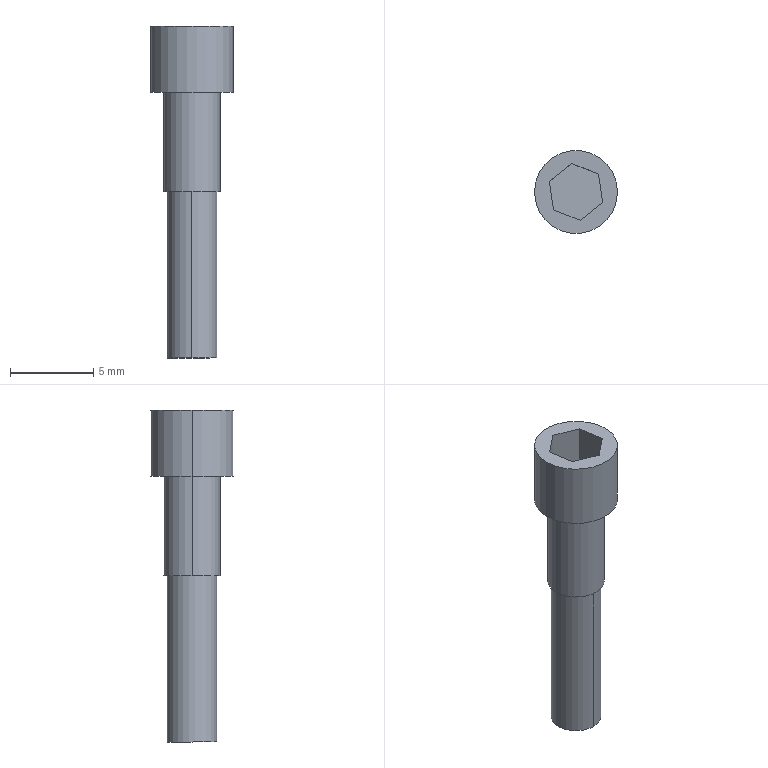Part | SolidWorks | features ICE 2, Cut 1, Extrusion 1 | 1 solid | 17 faces | box 5 x 5 x 19.999 mm | volume 180.305 mm3 | plane 11 | cylinder 6 | commonest cylinder face diameters 3 x2 3.4 x2 5 x2
STEP:
#1=CARTESIAN_POINT('',(2.5,-6.,4.));
#2=VERTEX_POINT('',#1);
#3=CARTESIAN_POINT('',(-2.5,-6.,4.));
#4=VERTEX_POINT('',#3);
#5=CARTESIAN_POINT('',(0.,-6.,4.));
#6=DIRECTION('',(0.,0.,1.));
#7=DIRECTION('',(1.,0.,0.));
#8=AXIS2_PLACEMENT_3D('',#5,#6,#7);
#9=CIRCLE('',#8,2.5);
#10=EDGE_CURVE('',#2,#4,#9,.T.);
#11=ORIENTED_EDGE('',*,*,#10,.F.);
#12=CARTESIAN_POINT('',(2.5,-6.,0.));
#13=VERTEX_POINT('',#12);
#14=CARTESIAN_POINT('',(2.5,-6.,4.));
#15=DIRECTION('',(0.,0.,-1.));
#16=VECTOR('',#15,1000.);
#17=LINE('',#14,#16);
#18=EDGE_CURVE('',#2,#13,#17,.T.);
#19=ORIENTED_EDGE('',*,*,#18,.T.);
#20=CARTESIAN_POINT('',(-2.5,-6.,0.));
#21=VERTEX_POINT('',#20);
#22=CARTESIAN_POINT('',(0.,-6.,0.));
#23=DIRECTION('',(0.,0.,1.));
#24=DIRECTION('',(1.,0.,0.));
#25=AXIS2_PLACEMENT_3D('',#22,#23,#24);
#26=CIRCLE('',#25,2.5);
#27=EDGE_CURVE('',#13,#21,#26,.T.);
#28=ORIENTED_EDGE('',*,*,#27,.T.);
#29=CARTESIAN_POINT('',(-2.5,-6.,4.));
#30=DIRECTION('',(0.,0.,-1.));
#31=VECTOR('',#30,1000.);
#32=LINE('',#29,#31);
#33=EDGE_CURVE('',#4,#21,#32,.T.);
#34=ORIENTED_EDGE('',*,*,#33,.F.);
#35=EDGE_LOOP('',(#11,#19,#28,#34));
#36=FACE_OUTER_BOUND('',#35,.T.);
#37=CARTESIAN_POINT('',(0.,-6.,4.));
#38=DIRECTION('',(0.,0.,-1.));
#39=DIRECTION('',(-1.,0.,0.));
#40=AXIS2_PLACEMENT_3D('',#37,#38,#39);
#41=CYLINDRICAL_SURFACE('',#40,2.5);
#42=ADVANCED_FACE('',(#36),#41,.T.);
#43=CARTESIAN_POINT('',(0.,-4.5,-15.999));
#44=VERTEX_POINT('',#43);
#45=CARTESIAN_POINT('',(0.,-7.5,-15.999));
#46=VERTEX_POINT('',#45);
#47=CARTESIAN_POINT('',(0.,-6.,-15.999));
#48=DIRECTION('',(0.,0.,-1.));
#49=DIRECTION('',(0.,1.,0.));
#50=AXIS2_PLACEMENT_3D('',#47,#48,#49);
#51=CIRCLE('',#50,1.5);
#52=EDGE_CURVE('',#44,#46,#51,.T.);
#53=ORIENTED_EDGE('',*,*,#52,.F.);
#54=CARTESIAN_POINT('',(0.,-4.5,-5.999));
#55=VERTEX_POINT('',#54);
#56=CARTESIAN_POINT('',(0.,-4.5,-20.241));
#57=DIRECTION('',(0.,0.,1.));
#58=VECTOR('',#57,1000.);
#59=LINE('',#56,#58);
#60=EDGE_CURVE('',#44,#55,#59,.T.);
#61=ORIENTED_EDGE('',*,*,#60,.T.);
#62=CARTESIAN_POINT('',(0.,-7.5,-5.999));
#63=VERTEX_POINT('',#62);
#64=CARTESIAN_POINT('',(0.,-6.,-5.999));
#65=DIRECTION('',(0.,0.,-1.));
#66=DIRECTION('',(0.,1.,0.));
#67=AXIS2_PLACEMENT_3D('',#64,#65,#66);
#68=CIRCLE('',#67,1.5);
#69=EDGE_CURVE('',#55,#63,#68,.T.);
#70=ORIENTED_EDGE('',*,*,#69,.T.);
#71=CARTESIAN_POINT('',(0.,-7.5,-20.241));
#72=DIRECTION('',(0.,0.,1.));
#73=VECTOR('',#72,1000.);
#74=LINE('',#71,#73);
#75=EDGE_CURVE('',#46,#63,#74,.T.);
#76=ORIENTED_EDGE('',*,*,#75,.F.);
#77=EDGE_LOOP('',(#53,#61,#70,#76));
#78=FACE_OUTER_BOUND('',#77,.T.);
#79=CARTESIAN_POINT('',(0.,-6.,-20.241));
#80=DIRECTION('',(0.,0.,1.));
#81=DIRECTION('',(0.,-1.,0.));
#82=AXIS2_PLACEMENT_3D('',#79,#80,#81);
#83=CYLINDRICAL_SURFACE('',#82,1.5);
#84=ADVANCED_FACE('',(#78),#83,.T.);
#85=CARTESIAN_POINT('',(1.7,-6.,-5.999));
#86=VERTEX_POINT('',#85);
#87=CARTESIAN_POINT('',(-1.7,-6.,-5.999));
#88=VERTEX_POINT('',#87);
#89=CARTESIAN_POINT('',(0.,-6.,-5.999));
#90=DIRECTION('',(0.,0.,1.));
#91=DIRECTION('',(0.,1.,0.));
#92=AXIS2_PLACEMENT_3D('',#89,#90,#91);
#93=CIRCLE('',#92,1.7);
#94=EDGE_CURVE('',#86,#88,#93,.T.);
#95=ORIENTED_EDGE('',*,*,#94,.T.);
#96=CARTESIAN_POINT('',(-1.7,-6.,0.));
#97=VERTEX_POINT('',#96);
#98=CARTESIAN_POINT('',(-1.7,-6.,-10.807));
#99=DIRECTION('',(0.,0.,1.));
#100=VECTOR('',#99,1000.);
#101=LINE('',#98,#100);
#102=EDGE_CURVE('',#88,#97,#101,.T.);
#103=ORIENTED_EDGE('',*,*,#102,.T.);
#104=CARTESIAN_POINT('',(1.7,-6.,0.));
#105=VERTEX_POINT('',#104);
#106=CARTESIAN_POINT('',(0.,-6.,0.));
#107=DIRECTION('',(0.,0.,1.));
#108=DIRECTION('',(1.,0.,0.));
#109=AXIS2_PLACEMENT_3D('',#106,#107,#108);
#110=CIRCLE('',#109,1.7);
#111=EDGE_CURVE('',#105,#97,#110,.T.);
#112=ORIENTED_EDGE('',*,*,#111,.F.);
#113=CARTESIAN_POINT('',(1.7,-6.,-10.807));
#114=DIRECTION('',(0.,0.,1.));
#115=VECTOR('',#114,1000.);
#116=LINE('',#113,#115);
#117=EDGE_CURVE('',#86,#105,#116,.T.);
#118=ORIENTED_EDGE('',*,*,#117,.F.);
#119=EDGE_LOOP('',(#95,#103,#112,#118));
#120=FACE_OUTER_BOUND('',#119,.T.);
#121=CARTESIAN_POINT('',(0.,-6.,-10.807));
#122=DIRECTION('',(0.,0.,1.));
#123=DIRECTION('',(1.,0.,0.));
#124=AXIS2_PLACEMENT_3D('',#121,#122,#123);
#125=CYLINDRICAL_SURFACE('',#124,1.7);
#126=ADVANCED_FACE('',(#120),#125,.T.);
#127=CARTESIAN_POINT('',(0.,-6.,-5.999));
#128=DIRECTION('',(0.,0.,-1.));
#129=DIRECTION('',(0.,1.,0.));
#130=AXIS2_PLACEMENT_3D('',#127,#128,#129);
#131=CIRCLE('',#130,1.5);
#132=EDGE_CURVE('',#63,#55,#131,.T.);
#133=ORIENTED_EDGE('',*,*,#132,.F.);
#134=ORIENTED_EDGE('',*,*,#69,.F.);
#135=EDGE_LOOP('',(#133,#134));
#136=FACE_BOUND('',#135,.T.);
#137=ORIENTED_EDGE('',*,*,#94,.F.);
#138=CARTESIAN_POINT('',(0.,-6.,-5.999));
#139=DIRECTION('',(0.,0.,1.));
#140=DIRECTION('',(0.,1.,0.));
#141=AXIS2_PLACEMENT_3D('',#138,#139,#140);
#142=CIRCLE('',#141,1.7);
#143=EDGE_CURVE('',#88,#86,#142,.T.);
#144=ORIENTED_EDGE('',*,*,#143,.F.);
#145=EDGE_LOOP('',(#137,#144));
#146=FACE_OUTER_BOUND('',#145,.T.);
#147=CARTESIAN_POINT('',(5.835,-7.398,-5.999));
#148=DIRECTION('',(0.,0.,-1.));
#149=DIRECTION('',(0.233,0.9725,0.));
#150=AXIS2_PLACEMENT_3D('',#147,#148,#149);
#151=PLANE('',#150);
#152=ADVANCED_FACE('',(#136,#146),#151,.T.);
#153=ORIENTED_EDGE('',*,*,#102,.F.);
#154=ORIENTED_EDGE('',*,*,#143,.T.);
#155=ORIENTED_EDGE('',*,*,#117,.T.);
#156=CARTESIAN_POINT('',(0.,-6.,0.));
#157=DIRECTION('',(0.,0.,1.));
#158=DIRECTION('',(1.,0.,0.));
#159=AXIS2_PLACEMENT_3D('',#156,#157,#158);
#160=CIRCLE('',#159,1.7);
#161=EDGE_CURVE('',#97,#105,#160,.T.);
#162=ORIENTED_EDGE('',*,*,#161,.F.);
#163=EDGE_LOOP('',(#153,#154,#155,#162));
#164=FACE_OUTER_BOUND('',#163,.T.);
#165=CARTESIAN_POINT('',(0.,-6.,-10.807));
#166=DIRECTION('',(0.,0.,1.));
#167=DIRECTION('',(1.,0.,0.));
#168=AXIS2_PLACEMENT_3D('',#165,#166,#167);
#169=CYLINDRICAL_SURFACE('',#168,1.7);
#170=ADVANCED_FACE('',(#164),#169,.T.);
#171=ORIENTED_EDGE('',*,*,#60,.F.);
#172=CARTESIAN_POINT('',(0.,-6.,-15.999));
#173=DIRECTION('',(0.,0.,-1.));
#174=DIRECTION('',(0.,1.,0.));
#175=AXIS2_PLACEMENT_3D('',#172,#173,#174);
#176=CIRCLE('',#175,1.5);
#177=EDGE_CURVE('',#46,#44,#176,.T.);
#178=ORIENTED_EDGE('',*,*,#177,.F.);
#179=ORIENTED_EDGE('',*,*,#75,.T.);
#180=ORIENTED_EDGE('',*,*,#132,.T.);
#181=EDGE_LOOP('',(#171,#178,#179,#180));
#182=FACE_OUTER_BOUND('',#181,.T.);
#183=CARTESIAN_POINT('',(0.,-6.,-20.241));
#184=DIRECTION('',(0.,0.,1.));
#185=DIRECTION('',(0.,-1.,0.));
#186=AXIS2_PLACEMENT_3D('',#183,#184,#185);
#187=CYLINDRICAL_SURFACE('',#186,1.5);
#188=ADVANCED_FACE('',(#182),#187,.T.);
#189=ORIENTED_EDGE('',*,*,#177,.T.);
#190=ORIENTED_EDGE('',*,*,#52,.T.);
#191=EDGE_LOOP('',(#189,#190));
#192=FACE_OUTER_BOUND('',#191,.T.);
#193=CARTESIAN_POINT('',(8.266,-7.981,-15.999));
#194=DIRECTION('',(0.,0.,-1.));
#195=DIRECTION('',(-0.9725,0.233,0.));
#196=AXIS2_PLACEMENT_3D('',#193,#194,#195);
#197=PLANE('',#196);
#198=ADVANCED_FACE('',(#192),#197,.T.);
#199=ORIENTED_EDGE('',*,*,#18,.F.);
#200=CARTESIAN_POINT('',(0.,-6.,4.));
#201=DIRECTION('',(0.,0.,1.));
#202=DIRECTION('',(1.,0.,0.));
#203=AXIS2_PLACEMENT_3D('',#200,#201,#202);
#204=CIRCLE('',#203,2.5);
#205=EDGE_CURVE('',#4,#2,#204,.T.);
#206=ORIENTED_EDGE('',*,*,#205,.F.);
#207=ORIENTED_EDGE('',*,*,#33,.T.);
#208=CARTESIAN_POINT('',(0.,-6.,0.));
#209=DIRECTION('',(0.,0.,1.));
#210=DIRECTION('',(1.,0.,0.));
#211=AXIS2_PLACEMENT_3D('',#208,#209,#210);
#212=CIRCLE('',#211,2.5);
#213=EDGE_CURVE('',#21,#13,#212,.T.);
#214=ORIENTED_EDGE('',*,*,#213,.T.);
#215=EDGE_LOOP('',(#199,#206,#207,#214));
#216=FACE_OUTER_BOUND('',#215,.T.);
#217=CARTESIAN_POINT('',(0.,-6.,4.));
#218=DIRECTION('',(0.,0.,-1.));
#219=DIRECTION('',(-1.,0.,0.));
#220=AXIS2_PLACEMENT_3D('',#217,#218,#219);
#221=CYLINDRICAL_SURFACE('',#220,2.5);
#222=ADVANCED_FACE('',(#216),#221,.T.);
#223=CARTESIAN_POINT('',(1.612,-6.635,4.));
#224=VERTEX_POINT('',#223);
#225=CARTESIAN_POINT('',(1.356,-4.922,4.));
#226=VERTEX_POINT('',#225);
#227=CARTESIAN_POINT('',(1.612,-6.635,4.));
#228=DIRECTION('',(-0.1478,0.989,0.));
#229=VECTOR('',#228,1000.);
#230=LINE('',#227,#229);
#231=EDGE_CURVE('',#224,#226,#230,.T.);
#232=ORIENTED_EDGE('',*,*,#231,.F.);
#233=CARTESIAN_POINT('',(0.256,-7.713,4.));
#234=VERTEX_POINT('',#233);
#235=CARTESIAN_POINT('',(0.256,-7.713,4.));
#236=DIRECTION('',(0.7826,0.6225,0.));
#237=VECTOR('',#236,1000.);
#238=LINE('',#235,#237);
#239=EDGE_CURVE('',#234,#224,#238,.T.);
#240=ORIENTED_EDGE('',*,*,#239,.F.);
#241=CARTESIAN_POINT('',(-1.356,-7.078,4.));
#242=VERTEX_POINT('',#241);
#243=CARTESIAN_POINT('',(-1.356,-7.078,4.));
#244=DIRECTION('',(0.9304,-0.3665,0.));
#245=VECTOR('',#244,1000.);
#246=LINE('',#243,#245);
#247=EDGE_CURVE('',#242,#234,#246,.T.);
#248=ORIENTED_EDGE('',*,*,#247,.F.);
#249=CARTESIAN_POINT('',(-1.612,-5.365,4.));
#250=VERTEX_POINT('',#249);
#251=CARTESIAN_POINT('',(-1.612,-5.365,4.));
#252=DIRECTION('',(0.1478,-0.989,0.));
#253=VECTOR('',#252,1000.);
#254=LINE('',#251,#253);
#255=EDGE_CURVE('',#250,#242,#254,.T.);
#256=ORIENTED_EDGE('',*,*,#255,.F.);
#257=CARTESIAN_POINT('',(-0.256,-4.287,4.));
#258=VERTEX_POINT('',#257);
#259=CARTESIAN_POINT('',(-0.256,-4.287,4.));
#260=DIRECTION('',(-0.7826,-0.6225,0.));
#261=VECTOR('',#260,1000.);
#262=LINE('',#259,#261);
#263=EDGE_CURVE('',#258,#250,#262,.T.);
#264=ORIENTED_EDGE('',*,*,#263,.F.);
#265=CARTESIAN_POINT('',(1.356,-4.922,4.));
#266=DIRECTION('',(-0.9304,0.3665,0.));
#267=VECTOR('',#266,1000.);
#268=LINE('',#265,#267);
#269=EDGE_CURVE('',#226,#258,#268,.T.);
#270=ORIENTED_EDGE('',*,*,#269,.F.);
#271=EDGE_LOOP('',(#232,#240,#248,#256,#264,#270));
#272=FACE_BOUND('',#271,.T.);
#273=ORIENTED_EDGE('',*,*,#205,.T.);
#274=ORIENTED_EDGE('',*,*,#10,.T.);
#275=EDGE_LOOP('',(#273,#274));
#276=FACE_OUTER_BOUND('',#275,.T.);
#277=CARTESIAN_POINT('',(0.,-6.,4.));
#278=DIRECTION('',(0.,0.,1.));
#279=DIRECTION('',(1.,0.,0.));
#280=AXIS2_PLACEMENT_3D('',#277,#278,#279);
#281=PLANE('',#280);
#282=ADVANCED_FACE('',(#272,#276),#281,.T.);
#283=ORIENTED_EDGE('',*,*,#111,.T.);
#284=ORIENTED_EDGE('',*,*,#161,.T.);
#285=EDGE_LOOP('',(#283,#284));
#286=FACE_BOUND('',#285,.T.);
#287=ORIENTED_EDGE('',*,*,#213,.F.);
#288=ORIENTED_EDGE('',*,*,#27,.F.);
#289=EDGE_LOOP('',(#287,#288));
#290=FACE_OUTER_BOUND('',#289,.T.);
#291=CARTESIAN_POINT('',(0.,-6.,0.));
#292=DIRECTION('',(0.,0.,1.));
#293=DIRECTION('',(1.,0.,0.));
#294=AXIS2_PLACEMENT_3D('',#291,#292,#293);
#295=PLANE('',#294);
#296=ADVANCED_FACE('',(#286,#290),#295,.F.);
#297=ORIENTED_EDGE('',*,*,#231,.T.);
#298=CARTESIAN_POINT('',(1.356,-4.922,1.));
#299=VERTEX_POINT('',#298);
#300=CARTESIAN_POINT('',(1.356,-4.922,1.));
#301=DIRECTION('',(0.,0.,1.));
#302=VECTOR('',#301,1000.);
#303=LINE('',#300,#302);
#304=EDGE_CURVE('',#299,#226,#303,.T.);
#305=ORIENTED_EDGE('',*,*,#304,.F.);
#306=CARTESIAN_POINT('',(1.612,-6.635,1.));
#307=VERTEX_POINT('',#306);
#308=CARTESIAN_POINT('',(1.612,-6.635,1.));
#309=DIRECTION('',(-0.1478,0.989,0.));
#310=VECTOR('',#309,1000.);
#311=LINE('',#308,#310);
#312=EDGE_CURVE('',#307,#299,#311,.T.);
#313=ORIENTED_EDGE('',*,*,#312,.F.);
#314=CARTESIAN_POINT('',(1.612,-6.635,1.));
#315=DIRECTION('',(0.,0.,1.));
#316=VECTOR('',#315,1000.);
#317=LINE('',#314,#316);
#318=EDGE_CURVE('',#307,#224,#317,.T.);
#319=ORIENTED_EDGE('',*,*,#318,.T.);
#320=EDGE_LOOP('',(#297,#305,#313,#319));
#321=FACE_OUTER_BOUND('',#320,.T.);
#322=CARTESIAN_POINT('',(1.612,-6.635,1.));
#323=DIRECTION('',(0.989,0.1478,0.));
#324=DIRECTION('',(-0.1478,0.989,0.));
#325=AXIS2_PLACEMENT_3D('',#322,#323,#324);
#326=PLANE('',#325);
#327=ADVANCED_FACE('',(#321),#326,.F.);
#328=ORIENTED_EDGE('',*,*,#239,.T.);
#329=ORIENTED_EDGE('',*,*,#318,.F.);
#330=CARTESIAN_POINT('',(0.256,-7.713,1.));
#331=VERTEX_POINT('',#330);
#332=CARTESIAN_POINT('',(0.256,-7.713,1.));
#333=DIRECTION('',(0.7826,0.6225,0.));
#334=VECTOR('',#333,1000.);
#335=LINE('',#332,#334);
#336=EDGE_CURVE('',#331,#307,#335,.T.);
#337=ORIENTED_EDGE('',*,*,#336,.F.);
#338=CARTESIAN_POINT('',(0.256,-7.713,1.));
#339=DIRECTION('',(0.,0.,1.));
#340=VECTOR('',#339,1000.);
#341=LINE('',#338,#340);
#342=EDGE_CURVE('',#331,#234,#341,.T.);
#343=ORIENTED_EDGE('',*,*,#342,.T.);
#344=EDGE_LOOP('',(#328,#329,#337,#343));
#345=FACE_OUTER_BOUND('',#344,.T.);
#346=CARTESIAN_POINT('',(0.256,-7.713,1.));
#347=DIRECTION('',(0.6225,-0.7826,0.));
#348=DIRECTION('',(0.7826,0.6225,0.));
#349=AXIS2_PLACEMENT_3D('',#346,#347,#348);
#350=PLANE('',#349);
#351=ADVANCED_FACE('',(#345),#350,.F.);
#352=ORIENTED_EDGE('',*,*,#247,.T.);
#353=ORIENTED_EDGE('',*,*,#342,.F.);
#354=CARTESIAN_POINT('',(-1.356,-7.078,1.));
#355=VERTEX_POINT('',#354);
#356=CARTESIAN_POINT('',(-1.356,-7.078,1.));
#357=DIRECTION('',(0.9304,-0.3665,0.));
#358=VECTOR('',#357,1000.);
#359=LINE('',#356,#358);
#360=EDGE_CURVE('',#355,#331,#359,.T.);
#361=ORIENTED_EDGE('',*,*,#360,.F.);
#362=CARTESIAN_POINT('',(-1.356,-7.078,1.));
#363=DIRECTION('',(0.,0.,1.));
#364=VECTOR('',#363,1000.);
#365=LINE('',#362,#364);
#366=EDGE_CURVE('',#355,#242,#365,.T.);
#367=ORIENTED_EDGE('',*,*,#366,.T.);
#368=EDGE_LOOP('',(#352,#353,#361,#367));
#369=FACE_OUTER_BOUND('',#368,.T.);
#370=CARTESIAN_POINT('',(-1.356,-7.078,1.));
#371=DIRECTION('',(-0.3665,-0.9304,0.));
#372=DIRECTION('',(0.9304,-0.3665,0.));
#373=AXIS2_PLACEMENT_3D('',#370,#371,#372);
#374=PLANE('',#373);
#375=ADVANCED_FACE('',(#369),#374,.F.);
#376=ORIENTED_EDGE('',*,*,#255,.T.);
#377=ORIENTED_EDGE('',*,*,#366,.F.);
#378=CARTESIAN_POINT('',(-1.612,-5.365,1.));
#379=VERTEX_POINT('',#378);
#380=CARTESIAN_POINT('',(-1.612,-5.365,1.));
#381=DIRECTION('',(0.1478,-0.989,0.));
#382=VECTOR('',#381,1000.);
#383=LINE('',#380,#382);
#384=EDGE_CURVE('',#379,#355,#383,.T.);
#385=ORIENTED_EDGE('',*,*,#384,.F.);
#386=CARTESIAN_POINT('',(-1.612,-5.365,1.));
#387=DIRECTION('',(0.,0.,1.));
#388=VECTOR('',#387,1000.);
#389=LINE('',#386,#388);
#390=EDGE_CURVE('',#379,#250,#389,.T.);
#391=ORIENTED_EDGE('',*,*,#390,.T.);
#392=EDGE_LOOP('',(#376,#377,#385,#391));
#393=FACE_OUTER_BOUND('',#392,.T.);
#394=CARTESIAN_POINT('',(-1.612,-5.365,1.));
#395=DIRECTION('',(-0.989,-0.1478,0.));
#396=DIRECTION('',(0.1478,-0.989,0.));
#397=AXIS2_PLACEMENT_3D('',#394,#395,#396);
#398=PLANE('',#397);
#399=ADVANCED_FACE('',(#393),#398,.F.);
#400=ORIENTED_EDGE('',*,*,#263,.T.);
#401=ORIENTED_EDGE('',*,*,#390,.F.);
#402=CARTESIAN_POINT('',(-0.256,-4.287,1.));
#403=VERTEX_POINT('',#402);
#404=CARTESIAN_POINT('',(-0.256,-4.287,1.));
#405=DIRECTION('',(-0.7826,-0.6225,0.));
#406=VECTOR('',#405,1000.);
#407=LINE('',#404,#406);
#408=EDGE_CURVE('',#403,#379,#407,.T.);
#409=ORIENTED_EDGE('',*,*,#408,.F.);
#410=CARTESIAN_POINT('',(-0.256,-4.287,1.));
#411=DIRECTION('',(0.,0.,1.));
#412=VECTOR('',#411,1000.);
#413=LINE('',#410,#412);
#414=EDGE_CURVE('',#403,#258,#413,.T.);
#415=ORIENTED_EDGE('',*,*,#414,.T.);
#416=EDGE_LOOP('',(#400,#401,#409,#415));
#417=FACE_OUTER_BOUND('',#416,.T.);
#418=CARTESIAN_POINT('',(-0.256,-4.287,1.));
#419=DIRECTION('',(-0.6225,0.7826,0.));
#420=DIRECTION('',(-0.7826,-0.6225,0.));
#421=AXIS2_PLACEMENT_3D('',#418,#419,#420);
#422=PLANE('',#421);
#423=ADVANCED_FACE('',(#417),#422,.F.);
#424=ORIENTED_EDGE('',*,*,#269,.T.);
#425=ORIENTED_EDGE('',*,*,#414,.F.);
#426=CARTESIAN_POINT('',(1.356,-4.922,1.));
#427=DIRECTION('',(-0.9304,0.3665,0.));
#428=VECTOR('',#427,1000.);
#429=LINE('',#426,#428);
#430=EDGE_CURVE('',#299,#403,#429,.T.);
#431=ORIENTED_EDGE('',*,*,#430,.F.);
#432=ORIENTED_EDGE('',*,*,#304,.T.);
#433=EDGE_LOOP('',(#424,#425,#431,#432));
#434=FACE_OUTER_BOUND('',#433,.T.);
#435=CARTESIAN_POINT('',(1.356,-4.922,1.));
#436=DIRECTION('',(0.3665,0.9304,0.));
#437=DIRECTION('',(-0.9304,0.3665,0.));
#438=AXIS2_PLACEMENT_3D('',#435,#436,#437);
#439=PLANE('',#438);
#440=ADVANCED_FACE('',(#434),#439,.F.);
#441=ORIENTED_EDGE('',*,*,#312,.T.);
#442=ORIENTED_EDGE('',*,*,#430,.T.);
#443=ORIENTED_EDGE('',*,*,#408,.T.);
#444=ORIENTED_EDGE('',*,*,#384,.T.);
#445=ORIENTED_EDGE('',*,*,#360,.T.);
#446=ORIENTED_EDGE('',*,*,#336,.T.);
#447=EDGE_LOOP('',(#441,#442,#443,#444,#445,#446));
#448=FACE_OUTER_BOUND('',#447,.T.);
#449=CARTESIAN_POINT('',(0.,0.,1.));
#450=DIRECTION('',(0.,0.,1.));
#451=DIRECTION('',(1.,0.,0.));
#452=AXIS2_PLACEMENT_3D('',#449,#450,#451);
#453=PLANE('',#452);
#454=ADVANCED_FACE('',(#448),#453,.T.);
#455=CLOSED_SHELL('',(#42,#84,#126,#152,#170,#188,#198,#222,#282,#296,#327,#351,#375,#399,#423,#440,#454));
#456=MANIFOLD_SOLID_BREP('',#455);
#457=CARTESIAN_POINT('',(0.,0.,0.));
#458=DIRECTION('',(0.,0.,1.));
#459=DIRECTION('',(1.,0.,0.));
#460=AXIS2_PLACEMENT_3D('',#457,#458,#459);
#461=(LENGTH_UNIT()NAMED_UNIT(*)SI_UNIT(.MILLI.,.METRE.));
#462=UNCERTAINTY_MEASURE_WITH_UNIT(LENGTH_MEASURE(0.00001),#461,'','');
#463=(NAMED_UNIT(*)PLANE_ANGLE_UNIT()SI_UNIT($,.RADIAN.));
#464=(NAMED_UNIT(*)SI_UNIT($,.STERADIAN.)SOLID_ANGLE_UNIT());
#465=(GEOMETRIC_REPRESENTATION_CONTEXT(3)GLOBAL_UNCERTAINTY_ASSIGNED_CONTEXT((#462))GLOBAL_UNIT_ASSIGNED_CONTEXT((#461,#463,#464))REPRESENTATION_CONTEXT('',''));
#466=ADVANCED_BREP_SHAPE_REPRESENTATION('',(#456,#460),#465);